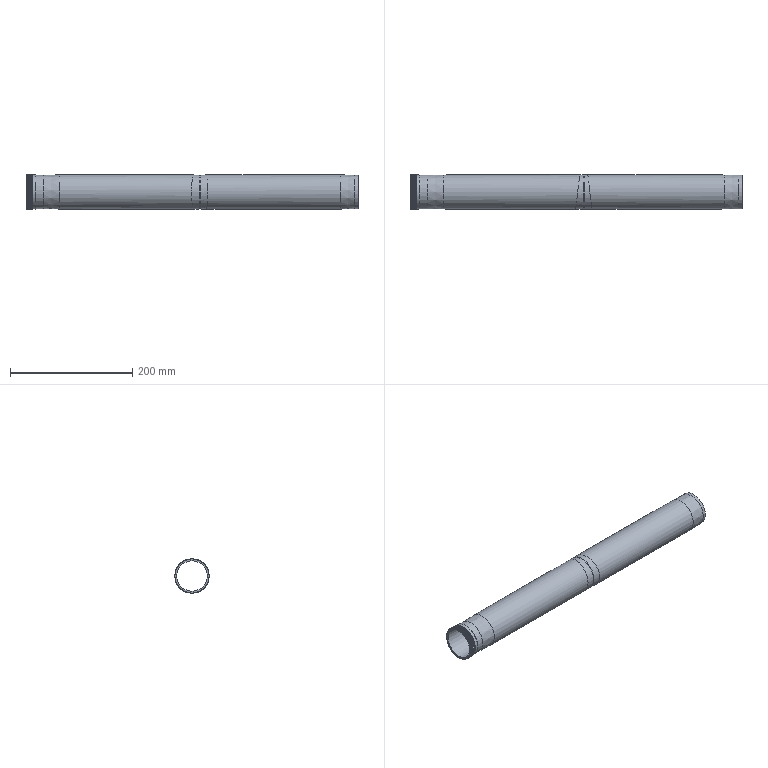Part | STEP file | PN_0023_default | 1 solid | 1364 faces | box 543 x 56 x 56 mm | volume 266273 mm3 | plane 1353 | cylinder 9 | cone 2 | commonest cylinder face diameters 56 x6 50 x1 54.628 x1 54.754 x1